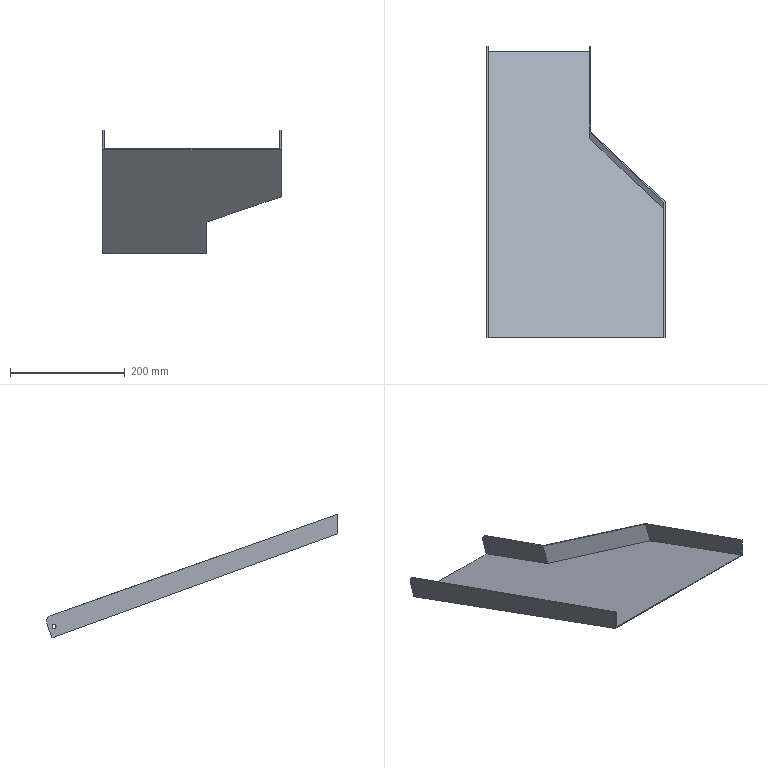Part | NX | features HB 2 | 1 solid | 18 faces | box 311 x 508.386 x 215.484 mm | volume 344938 mm3 | plane 14 | cylinder 4 | commonest cylinder face diameters 7 x2 20 x2
STEP:
#1=CARTESIAN_POINT('',(3094.,539.252,-364.707));
#2=VERTEX_POINT('',#1);
#3=CARTESIAN_POINT('',(3094.,691.161,-419.998));
#4=VERTEX_POINT('',#3);
#5=CARTESIAN_POINT('',(3094.,379.611,-306.603));
#6=DIRECTION('',(0.,0.9397,-0.342));
#7=VECTOR('',#6,1000.);
#8=LINE('',#5,#7);
#9=EDGE_CURVE('',#2,#4,#8,.T.);
#10=ORIENTED_EDGE('',*,*,#9,.T.);
#11=CARTESIAN_POINT('',(2917.,691.161,-419.998));
#12=VERTEX_POINT('',#11);
#13=CARTESIAN_POINT('',(2992.,691.161,-419.998));
#14=DIRECTION('',(1.,0.,0.));
#15=VECTOR('',#14,1000.);
#16=LINE('',#13,#15);
#17=EDGE_CURVE('',#12,#4,#16,.T.);
#18=ORIENTED_EDGE('',*,*,#17,.F.);
#19=CARTESIAN_POINT('',(2917.,192.,-238.318));
#20=VERTEX_POINT('',#19);
#21=CARTESIAN_POINT('',(2917.,379.611,-306.603));
#22=DIRECTION('',(0.,-0.9397,0.342));
#23=VECTOR('',#22,1000.);
#24=LINE('',#21,#23);
#25=EDGE_CURVE('',#12,#20,#24,.T.);
#26=ORIENTED_EDGE('',*,*,#25,.T.);
#27=CARTESIAN_POINT('',(3224.,192.,-238.318));
#28=VERTEX_POINT('',#27);
#29=CARTESIAN_POINT('',(2992.,192.,-238.318));
#30=DIRECTION('',(-1.,0.,0.));
#31=VECTOR('',#30,1000.);
#32=LINE('',#29,#31);
#33=EDGE_CURVE('',#28,#20,#32,.T.);
#34=ORIENTED_EDGE('',*,*,#33,.F.);
#35=CARTESIAN_POINT('',(3224.,417.092,-320.245));
#36=VERTEX_POINT('',#35);
#37=CARTESIAN_POINT('',(3224.,379.611,-306.603));
#38=DIRECTION('',(0.,0.9397,-0.342));
#39=VECTOR('',#38,1000.);
#40=LINE('',#37,#39);
#41=EDGE_CURVE('',#28,#36,#40,.T.);
#42=ORIENTED_EDGE('',*,*,#41,.T.);
#43=CARTESIAN_POINT('',(3127.943,507.356,-353.098));
#44=DIRECTION('',(-0.7071,0.6645,-0.2418));
#45=VECTOR('',#44,1000.);
#46=LINE('',#43,#45);
#47=EDGE_CURVE('',#36,#2,#46,.T.);
#48=ORIENTED_EDGE('',*,*,#47,.T.);
#49=EDGE_LOOP('',(#10,#18,#26,#34,#42,#48));
#50=FACE_BOUND('',#49,.T.);
#51=CARTESIAN_POINT('',(2992.,379.611,-306.603));
#52=DIRECTION('',(0.,0.342,0.9397));
#53=DIRECTION('',(1.,0.,0.));
#54=AXIS2_PLACEMENT_3D('',#51,#52,#53);
#55=PLANE('',#54);
#56=ADVANCED_FACE('',(#50),#55,.T.);
#57=ORIENTED_EDGE('',*,*,#33,.T.);
#58=CARTESIAN_POINT('',(2917.,192.,-206.393));
#59=VERTEX_POINT('',#58);
#60=CARTESIAN_POINT('',(2917.,192.,-306.603));
#61=DIRECTION('',(0.,0.,1.));
#62=VECTOR('',#61,1000.);
#63=LINE('',#60,#62);
#64=EDGE_CURVE('',#20,#59,#63,.T.);
#65=ORIENTED_EDGE('',*,*,#64,.T.);
#66=CARTESIAN_POINT('',(2915.,192.,-206.393));
#67=VERTEX_POINT('',#66);
#68=CARTESIAN_POINT('',(3433.,192.,-206.393));
#69=DIRECTION('',(1.,0.,0.));
#70=VECTOR('',#69,1000.);
#71=LINE('',#68,#70);
#72=EDGE_CURVE('',#67,#59,#71,.T.);
#73=ORIENTED_EDGE('',*,*,#72,.F.);
#74=CARTESIAN_POINT('',(2915.,192.,-240.446));
#75=VERTEX_POINT('',#74);
#76=CARTESIAN_POINT('',(2915.,192.,-306.603));
#77=DIRECTION('',(0.,0.,1.));
#78=VECTOR('',#77,1000.);
#79=LINE('',#76,#78);
#80=EDGE_CURVE('',#75,#67,#79,.T.);
#81=ORIENTED_EDGE('',*,*,#80,.F.);
#82=CARTESIAN_POINT('',(3226.,192.,-240.446));
#83=VERTEX_POINT('',#82);
#84=CARTESIAN_POINT('',(2992.,192.,-240.446));
#85=DIRECTION('',(-1.,0.,0.));
#86=VECTOR('',#85,1000.);
#87=LINE('',#84,#86);
#88=EDGE_CURVE('',#83,#75,#87,.T.);
#89=ORIENTED_EDGE('',*,*,#88,.F.);
#90=CARTESIAN_POINT('',(3226.,192.,-206.393));
#91=VERTEX_POINT('',#90);
#92=CARTESIAN_POINT('',(3226.,192.,-306.603));
#93=DIRECTION('',(0.,0.,-1.));
#94=VECTOR('',#93,1000.);
#95=LINE('',#92,#94);
#96=EDGE_CURVE('',#91,#83,#95,.T.);
#97=ORIENTED_EDGE('',*,*,#96,.F.);
#98=CARTESIAN_POINT('',(3224.,192.,-206.393));
#99=VERTEX_POINT('',#98);
#100=CARTESIAN_POINT('',(3433.,192.,-206.393));
#101=DIRECTION('',(1.,0.,0.));
#102=VECTOR('',#101,1000.);
#103=LINE('',#100,#102);
#104=EDGE_CURVE('',#99,#91,#103,.T.);
#105=ORIENTED_EDGE('',*,*,#104,.F.);
#106=CARTESIAN_POINT('',(3224.,192.,-306.603));
#107=DIRECTION('',(0.,0.,-1.));
#108=VECTOR('',#107,1000.);
#109=LINE('',#106,#108);
#110=EDGE_CURVE('',#99,#28,#109,.T.);
#111=ORIENTED_EDGE('',*,*,#110,.T.);
#112=EDGE_LOOP('',(#57,#65,#73,#81,#89,#97,#105,#111));
#113=FACE_BOUND('',#112,.T.);
#114=CARTESIAN_POINT('',(3433.,192.,70.));
#115=DIRECTION('',(0.,-1.,0.));
#116=DIRECTION('',(0.,0.,-1.));
#117=AXIS2_PLACEMENT_3D('',#114,#115,#116);
#118=PLANE('',#117);
#119=ADVANCED_FACE('',(#113),#118,.T.);
#120=CARTESIAN_POINT('',(3226.,417.186,-322.407));
#121=VERTEX_POINT('',#120);
#122=CARTESIAN_POINT('',(3096.,539.346,-366.87));
#123=VERTEX_POINT('',#122);
#124=CARTESIAN_POINT('',(3129.357,508.001,-355.461));
#125=DIRECTION('',(-0.7071,0.6645,-0.2418));
#126=VECTOR('',#125,1000.);
#127=LINE('',#124,#126);
#128=EDGE_CURVE('',#121,#123,#127,.T.);
#129=ORIENTED_EDGE('',*,*,#128,.F.);
#130=CARTESIAN_POINT('',(3226.,378.927,-308.482));
#131=DIRECTION('',(0.,-0.9397,0.342));
#132=VECTOR('',#131,1000.);
#133=LINE('',#130,#132);
#134=EDGE_CURVE('',#121,#83,#133,.T.);
#135=ORIENTED_EDGE('',*,*,#134,.T.);
#136=ORIENTED_EDGE('',*,*,#88,.T.);
#137=CARTESIAN_POINT('',(2915.,690.477,-421.877));
#138=VERTEX_POINT('',#137);
#139=CARTESIAN_POINT('',(2915.,378.927,-308.482));
#140=DIRECTION('',(0.,0.9397,-0.342));
#141=VECTOR('',#140,1000.);
#142=LINE('',#139,#141);
#143=EDGE_CURVE('',#75,#138,#142,.T.);
#144=ORIENTED_EDGE('',*,*,#143,.T.);
#145=CARTESIAN_POINT('',(3096.,690.477,-421.877));
#146=VERTEX_POINT('',#145);
#147=CARTESIAN_POINT('',(2992.,690.477,-421.877));
#148=DIRECTION('',(1.,0.,0.));
#149=VECTOR('',#148,1000.);
#150=LINE('',#147,#149);
#151=EDGE_CURVE('',#138,#146,#150,.T.);
#152=ORIENTED_EDGE('',*,*,#151,.T.);
#153=CARTESIAN_POINT('',(3096.,378.927,-308.482));
#154=DIRECTION('',(0.,-0.9397,0.342));
#155=VECTOR('',#154,1000.);
#156=LINE('',#153,#155);
#157=EDGE_CURVE('',#146,#123,#156,.T.);
#158=ORIENTED_EDGE('',*,*,#157,.T.);
#159=EDGE_LOOP('',(#129,#135,#136,#144,#152,#158));
#160=FACE_BOUND('',#159,.T.);
#161=CARTESIAN_POINT('',(2992.,378.927,-308.482));
#162=DIRECTION('',(0.,0.342,0.9397));
#163=DIRECTION('',(1.,0.,0.));
#164=AXIS2_PLACEMENT_3D('',#161,#162,#163);
#165=PLANE('',#164);
#166=ADVANCED_FACE('',(#160),#165,.F.);
#167=CARTESIAN_POINT('',(2915.,693.714,-383.458));
#168=VERTEX_POINT('',#167);
#169=CARTESIAN_POINT('',(2915.,390.558,-276.468));
#170=DIRECTION('',(0.,-0.943,0.3328));
#171=VECTOR('',#170,1000.);
#172=LINE('',#169,#171);
#173=EDGE_CURVE('',#168,#67,#172,.T.);
#174=ORIENTED_EDGE('',*,*,#173,.T.);
#175=ORIENTED_EDGE('',*,*,#72,.T.);
#176=CARTESIAN_POINT('',(2917.,693.714,-383.458));
#177=VERTEX_POINT('',#176);
#178=CARTESIAN_POINT('',(2917.,390.558,-276.468));
#179=DIRECTION('',(0.,-0.943,0.3328));
#180=VECTOR('',#179,1000.);
#181=LINE('',#178,#180);
#182=EDGE_CURVE('',#177,#59,#181,.T.);
#183=ORIENTED_EDGE('',*,*,#182,.F.);
#184=CARTESIAN_POINT('',(2992.,693.714,-383.458));
#185=DIRECTION('',(1.,0.,0.));
#186=VECTOR('',#185,1000.);
#187=LINE('',#184,#186);
#188=EDGE_CURVE('',#168,#177,#187,.T.);
#189=ORIENTED_EDGE('',*,*,#188,.F.);
#190=EDGE_LOOP('',(#174,#175,#183,#189));
#191=FACE_BOUND('',#190,.T.);
#192=CARTESIAN_POINT('',(2927.,390.558,-276.468));
#193=DIRECTION('',(0.,-0.3328,-0.943));
#194=DIRECTION('',(0.,0.943,-0.3328));
#195=AXIS2_PLACEMENT_3D('',#192,#193,#194);
#196=PLANE('',#195);
#197=ADVANCED_FACE('',(#191),#196,.F.);
#198=ORIENTED_EDGE('',*,*,#182,.T.);
#199=ORIENTED_EDGE('',*,*,#64,.F.);
#200=ORIENTED_EDGE('',*,*,#25,.F.);
#201=CARTESIAN_POINT('',(2917.,699.783,-396.309));
#202=VERTEX_POINT('',#201);
#203=CARTESIAN_POINT('',(2917.,692.943,-415.102));
#204=DIRECTION('',(0.,0.342,0.9397));
#205=VECTOR('',#204,1000.);
#206=LINE('',#203,#205);
#207=EDGE_CURVE('',#12,#202,#206,.T.);
#208=ORIENTED_EDGE('',*,*,#207,.T.);
#209=CARTESIAN_POINT('',(2917.,690.386,-392.888));
#210=DIRECTION('',(-1.,0.,0.));
#211=DIRECTION('',(0.,0.,-1.));
#212=AXIS2_PLACEMENT_3D('',#209,#210,#211);
#213=CIRCLE('',#212,10.);
#214=EDGE_CURVE('',#177,#202,#213,.T.);
#215=ORIENTED_EDGE('',*,*,#214,.F.);
#216=EDGE_LOOP('',(#198,#199,#200,#208,#215));
#217=FACE_BOUND('',#216,.T.);
#218=CARTESIAN_POINT('',(2917.,686.661,-398.799));
#219=VERTEX_POINT('',#218);
#220=CARTESIAN_POINT('',(2917.,686.966,-402.285));
#221=DIRECTION('',(1.,0.,0.));
#222=DIRECTION('',(0.,-0.08716,0.9962));
#223=AXIS2_PLACEMENT_3D('',#220,#221,#222);
#224=CIRCLE('',#223,3.5);
#225=EDGE_CURVE('',#219,#219,#224,.T.);
#226=ORIENTED_EDGE('',*,*,#225,.F.);
#227=EDGE_LOOP('',(#226));
#228=FACE_BOUND('',#227,.T.);
#229=CARTESIAN_POINT('',(2917.,379.611,-306.603));
#230=DIRECTION('',(1.,0.,0.));
#231=DIRECTION('',(0.,-0.08716,0.9962));
#232=AXIS2_PLACEMENT_3D('',#229,#230,#231);
#233=PLANE('',#232);
#234=ADVANCED_FACE('',(#217,#228),#233,.T.);
#235=CARTESIAN_POINT('',(3096.,551.568,-333.292));
#236=VERTEX_POINT('',#235);
#237=CARTESIAN_POINT('',(3226.,428.973,-290.025));
#238=VERTEX_POINT('',#237);
#239=CARTESIAN_POINT('',(3226.012,428.961,-290.021));
#240=DIRECTION('',(0.7071,-0.6668,0.2353));
#241=VECTOR('',#240,1000.);
#242=LINE('',#239,#241);
#243=EDGE_CURVE('',#236,#238,#242,.T.);
#244=ORIENTED_EDGE('',*,*,#243,.F.);
#245=CARTESIAN_POINT('',(3096.,693.714,-383.458));
#246=VERTEX_POINT('',#245);
#247=CARTESIAN_POINT('',(3096.,390.558,-276.468));
#248=DIRECTION('',(0.,-0.943,0.3328));
#249=VECTOR('',#248,1000.);
#250=LINE('',#247,#249);
#251=EDGE_CURVE('',#246,#236,#250,.T.);
#252=ORIENTED_EDGE('',*,*,#251,.F.);
#253=CARTESIAN_POINT('',(3094.,693.714,-383.458));
#254=VERTEX_POINT('',#253);
#255=CARTESIAN_POINT('',(3224.,693.714,-383.458));
#256=DIRECTION('',(1.,0.,0.));
#257=VECTOR('',#256,1000.);
#258=LINE('',#255,#257);
#259=EDGE_CURVE('',#254,#246,#258,.T.);
#260=ORIENTED_EDGE('',*,*,#259,.F.);
#261=CARTESIAN_POINT('',(3094.,550.787,-333.016));
#262=VERTEX_POINT('',#261);
#263=CARTESIAN_POINT('',(3094.,390.558,-276.468));
#264=DIRECTION('',(0.,-0.943,0.3328));
#265=VECTOR('',#264,1000.);
#266=LINE('',#263,#265);
#267=EDGE_CURVE('',#254,#262,#266,.T.);
#268=ORIENTED_EDGE('',*,*,#267,.T.);
#269=CARTESIAN_POINT('',(3224.,428.191,-289.75));
#270=VERTEX_POINT('',#269);
#271=CARTESIAN_POINT('',(3224.598,427.628,-289.551));
#272=DIRECTION('',(0.7071,-0.6668,0.2353));
#273=VECTOR('',#272,1000.);
#274=LINE('',#271,#273);
#275=EDGE_CURVE('',#262,#270,#274,.T.);
#276=ORIENTED_EDGE('',*,*,#275,.T.);
#277=CARTESIAN_POINT('',(3224.,390.558,-276.468));
#278=DIRECTION('',(0.,-0.943,0.3328));
#279=VECTOR('',#278,1000.);
#280=LINE('',#277,#279);
#281=EDGE_CURVE('',#270,#99,#280,.T.);
#282=ORIENTED_EDGE('',*,*,#281,.T.);
#283=ORIENTED_EDGE('',*,*,#104,.T.);
#284=CARTESIAN_POINT('',(3226.,390.558,-276.468));
#285=DIRECTION('',(0.,-0.943,0.3328));
#286=VECTOR('',#285,1000.);
#287=LINE('',#284,#286);
#288=EDGE_CURVE('',#238,#91,#287,.T.);
#289=ORIENTED_EDGE('',*,*,#288,.F.);
#290=EDGE_LOOP('',(#244,#252,#260,#268,#276,#282,#283,#289));
#291=FACE_BOUND('',#290,.T.);
#292=CARTESIAN_POINT('',(3224.,390.558,-276.468));
#293=DIRECTION('',(0.,-0.3328,-0.943));
#294=DIRECTION('',(0.,0.943,-0.3328));
#295=AXIS2_PLACEMENT_3D('',#292,#293,#294);
#296=PLANE('',#295);
#297=ADVANCED_FACE('',(#291),#296,.F.);
#298=CARTESIAN_POINT('',(3224.,417.092,-320.245));
#299=DIRECTION('',(0.,-0.342,-0.9397));
#300=VECTOR('',#299,1000.);
#301=LINE('',#298,#300);
#302=EDGE_CURVE('',#270,#36,#301,.T.);
#303=ORIENTED_EDGE('',*,*,#302,.T.);
#304=ORIENTED_EDGE('',*,*,#41,.F.);
#305=ORIENTED_EDGE('',*,*,#110,.F.);
#306=ORIENTED_EDGE('',*,*,#281,.F.);
#307=EDGE_LOOP('',(#303,#304,#305,#306));
#308=FACE_BOUND('',#307,.T.);
#309=CARTESIAN_POINT('',(3224.,379.611,-306.603));
#310=DIRECTION('',(-1.,0.,0.));
#311=DIRECTION('',(0.,-0.08716,0.9962));
#312=AXIS2_PLACEMENT_3D('',#309,#310,#311);
#313=PLANE('',#312);
#314=ADVANCED_FACE('',(#308),#313,.T.);
#315=ORIENTED_EDGE('',*,*,#288,.T.);
#316=ORIENTED_EDGE('',*,*,#96,.T.);
#317=ORIENTED_EDGE('',*,*,#134,.F.);
#318=CARTESIAN_POINT('',(3226.,417.87,-320.528));
#319=DIRECTION('',(0.,0.342,0.9397));
#320=VECTOR('',#319,1000.);
#321=LINE('',#318,#320);
#322=EDGE_CURVE('',#121,#238,#321,.T.);
#323=ORIENTED_EDGE('',*,*,#322,.T.);
#324=EDGE_LOOP('',(#315,#316,#317,#323));
#325=FACE_BOUND('',#324,.T.);
#326=CARTESIAN_POINT('',(3226.,379.611,-306.603));
#327=DIRECTION('',(-1.,0.,0.));
#328=DIRECTION('',(0.,-0.08716,0.9962));
#329=AXIS2_PLACEMENT_3D('',#326,#327,#328);
#330=PLANE('',#329);
#331=ADVANCED_FACE('',(#325),#330,.F.);
#332=ORIENTED_EDGE('',*,*,#143,.F.);
#333=ORIENTED_EDGE('',*,*,#80,.T.);
#334=ORIENTED_EDGE('',*,*,#173,.F.);
#335=CARTESIAN_POINT('',(2915.,699.783,-396.309));
#336=VERTEX_POINT('',#335);
#337=CARTESIAN_POINT('',(2915.,690.386,-392.888));
#338=DIRECTION('',(1.,0.,0.));
#339=DIRECTION('',(0.,0.,-1.));
#340=AXIS2_PLACEMENT_3D('',#337,#338,#339);
#341=CIRCLE('',#340,10.);
#342=EDGE_CURVE('',#336,#168,#341,.T.);
#343=ORIENTED_EDGE('',*,*,#342,.F.);
#344=CARTESIAN_POINT('',(2915.,692.943,-415.102));
#345=DIRECTION('',(0.,0.342,0.9397));
#346=VECTOR('',#345,1000.);
#347=LINE('',#344,#346);
#348=EDGE_CURVE('',#138,#336,#347,.T.);
#349=ORIENTED_EDGE('',*,*,#348,.F.);
#350=EDGE_LOOP('',(#332,#333,#334,#343,#349));
#351=FACE_BOUND('',#350,.T.);
#352=CARTESIAN_POINT('',(2915.,686.661,-398.799));
#353=VERTEX_POINT('',#352);
#354=CARTESIAN_POINT('',(2915.,686.966,-402.285));
#355=DIRECTION('',(1.,0.,0.));
#356=DIRECTION('',(0.,-0.08716,0.9962));
#357=AXIS2_PLACEMENT_3D('',#354,#355,#356);
#358=CIRCLE('',#357,3.5);
#359=EDGE_CURVE('',#353,#353,#358,.T.);
#360=ORIENTED_EDGE('',*,*,#359,.T.);
#361=EDGE_LOOP('',(#360));
#362=FACE_BOUND('',#361,.T.);
#363=CARTESIAN_POINT('',(2915.,379.611,-306.603));
#364=DIRECTION('',(1.,0.,0.));
#365=DIRECTION('',(0.,0.08716,-0.9962));
#366=AXIS2_PLACEMENT_3D('',#363,#364,#365);
#367=PLANE('',#366);
#368=ADVANCED_FACE('',(#351,#362),#367,.F.);
#369=CARTESIAN_POINT('',(3096.,687.271,-405.772));
#370=VERTEX_POINT('',#369);
#371=CARTESIAN_POINT('',(3096.,686.966,-402.285));
#372=DIRECTION('',(1.,0.,0.));
#373=DIRECTION('',(0.,0.08716,-0.9962));
#374=AXIS2_PLACEMENT_3D('',#371,#372,#373);
#375=CIRCLE('',#374,3.5);
#376=EDGE_CURVE('',#370,#370,#375,.T.);
#377=ORIENTED_EDGE('',*,*,#376,.F.);
#378=EDGE_LOOP('',(#377));
#379=FACE_BOUND('',#378,.T.);
#380=ORIENTED_EDGE('',*,*,#157,.F.);
#381=CARTESIAN_POINT('',(3096.,699.783,-396.309));
#382=VERTEX_POINT('',#381);
#383=CARTESIAN_POINT('',(3096.,692.943,-415.102));
#384=DIRECTION('',(0.,0.342,0.9397));
#385=VECTOR('',#384,1000.);
#386=LINE('',#383,#385);
#387=EDGE_CURVE('',#146,#382,#386,.T.);
#388=ORIENTED_EDGE('',*,*,#387,.T.);
#389=CARTESIAN_POINT('',(3096.,690.386,-392.888));
#390=DIRECTION('',(-1.,0.,0.));
#391=DIRECTION('',(0.,0.,1.));
#392=AXIS2_PLACEMENT_3D('',#389,#390,#391);
#393=CIRCLE('',#392,10.);
#394=EDGE_CURVE('',#246,#382,#393,.T.);
#395=ORIENTED_EDGE('',*,*,#394,.F.);
#396=ORIENTED_EDGE('',*,*,#251,.T.);
#397=CARTESIAN_POINT('',(3096.,540.03,-364.991));
#398=DIRECTION('',(0.,0.342,0.9397));
#399=VECTOR('',#398,1000.);
#400=LINE('',#397,#399);
#401=EDGE_CURVE('',#123,#236,#400,.T.);
#402=ORIENTED_EDGE('',*,*,#401,.F.);
#403=EDGE_LOOP('',(#380,#388,#395,#396,#402));
#404=FACE_BOUND('',#403,.T.);
#405=CARTESIAN_POINT('',(3096.,379.611,-306.603));
#406=DIRECTION('',(-1.,0.,0.));
#407=DIRECTION('',(0.,-0.08716,0.9962));
#408=AXIS2_PLACEMENT_3D('',#405,#406,#407);
#409=PLANE('',#408);
#410=ADVANCED_FACE('',(#379,#404),#409,.F.);
#411=CARTESIAN_POINT('',(3094.,687.271,-405.772));
#412=VERTEX_POINT('',#411);
#413=CARTESIAN_POINT('',(3094.,686.966,-402.285));
#414=DIRECTION('',(-1.,0.,0.));
#415=DIRECTION('',(0.,0.08716,-0.9962));
#416=AXIS2_PLACEMENT_3D('',#413,#414,#415);
#417=CIRCLE('',#416,3.5);
#418=EDGE_CURVE('',#412,#412,#417,.T.);
#419=ORIENTED_EDGE('',*,*,#418,.F.);
#420=EDGE_LOOP('',(#419));
#421=FACE_BOUND('',#420,.T.);
#422=ORIENTED_EDGE('',*,*,#267,.F.);
#423=CARTESIAN_POINT('',(3094.,699.783,-396.309));
#424=VERTEX_POINT('',#423);
#425=CARTESIAN_POINT('',(3094.,690.386,-392.888));
#426=DIRECTION('',(1.,0.,0.));
#427=DIRECTION('',(0.,0.,1.));
#428=AXIS2_PLACEMENT_3D('',#425,#426,#427);
#429=CIRCLE('',#428,10.);
#430=EDGE_CURVE('',#424,#254,#429,.T.);
#431=ORIENTED_EDGE('',*,*,#430,.F.);
#432=CARTESIAN_POINT('',(3094.,692.943,-415.102));
#433=DIRECTION('',(0.,0.342,0.9397));
#434=VECTOR('',#433,1000.);
#435=LINE('',#432,#434);
#436=EDGE_CURVE('',#4,#424,#435,.T.);
#437=ORIENTED_EDGE('',*,*,#436,.F.);
#438=ORIENTED_EDGE('',*,*,#9,.F.);
#439=CARTESIAN_POINT('',(3094.,539.252,-364.707));
#440=DIRECTION('',(0.,0.342,0.9397));
#441=VECTOR('',#440,1000.);
#442=LINE('',#439,#441);
#443=EDGE_CURVE('',#2,#262,#442,.T.);
#444=ORIENTED_EDGE('',*,*,#443,.T.);
#445=EDGE_LOOP('',(#422,#431,#437,#438,#444));
#446=FACE_BOUND('',#445,.T.);
#447=CARTESIAN_POINT('',(3094.,379.611,-306.603));
#448=DIRECTION('',(-1.,0.,0.));
#449=DIRECTION('',(0.,-0.08716,0.9962));
#450=AXIS2_PLACEMENT_3D('',#447,#448,#449);
#451=PLANE('',#450);
#452=ADVANCED_FACE('',(#421,#446),#451,.T.);
#453=ORIENTED_EDGE('',*,*,#348,.T.);
#454=CARTESIAN_POINT('',(2992.,699.783,-396.309));
#455=DIRECTION('',(-1.,0.,0.));
#456=VECTOR('',#455,1000.);
#457=LINE('',#454,#456);
#458=EDGE_CURVE('',#202,#336,#457,.T.);
#459=ORIENTED_EDGE('',*,*,#458,.F.);
#460=ORIENTED_EDGE('',*,*,#207,.F.);
#461=ORIENTED_EDGE('',*,*,#17,.T.);
#462=ORIENTED_EDGE('',*,*,#436,.T.);
#463=CARTESIAN_POINT('',(3224.,699.783,-396.309));
#464=DIRECTION('',(-1.,0.,0.));
#465=VECTOR('',#464,1000.);
#466=LINE('',#463,#465);
#467=EDGE_CURVE('',#382,#424,#466,.T.);
#468=ORIENTED_EDGE('',*,*,#467,.F.);
#469=ORIENTED_EDGE('',*,*,#387,.F.);
#470=ORIENTED_EDGE('',*,*,#151,.F.);
#471=EDGE_LOOP('',(#453,#459,#460,#461,#462,#468,#469,#470));
#472=FACE_BOUND('',#471,.T.);
#473=CARTESIAN_POINT('',(2992.,692.943,-415.102));
#474=DIRECTION('',(0.,-0.9397,0.342));
#475=DIRECTION('',(0.,-0.342,-0.9397));
#476=AXIS2_PLACEMENT_3D('',#473,#474,#475);
#477=PLANE('',#476);
#478=ADVANCED_FACE('',(#472),#477,.F.);
#479=ORIENTED_EDGE('',*,*,#214,.T.);
#480=ORIENTED_EDGE('',*,*,#458,.T.);
#481=ORIENTED_EDGE('',*,*,#342,.T.);
#482=ORIENTED_EDGE('',*,*,#188,.T.);
#483=EDGE_LOOP('',(#479,#480,#481,#482));
#484=FACE_BOUND('',#483,.T.);
#485=CARTESIAN_POINT('',(2992.,690.386,-392.888));
#486=DIRECTION('',(1.,0.,0.));
#487=DIRECTION('',(0.,0.,1.));
#488=AXIS2_PLACEMENT_3D('',#485,#486,#487);
#489=CYLINDRICAL_SURFACE('',#488,10.);
#490=ADVANCED_FACE('',(#484),#489,.T.);
#491=ORIENTED_EDGE('',*,*,#430,.T.);
#492=ORIENTED_EDGE('',*,*,#259,.T.);
#493=ORIENTED_EDGE('',*,*,#394,.T.);
#494=ORIENTED_EDGE('',*,*,#467,.T.);
#495=EDGE_LOOP('',(#491,#492,#493,#494));
#496=FACE_BOUND('',#495,.T.);
#497=CARTESIAN_POINT('',(3224.,690.386,-392.888));
#498=DIRECTION('',(-1.,0.,0.));
#499=DIRECTION('',(0.,0.,-1.));
#500=AXIS2_PLACEMENT_3D('',#497,#498,#499);
#501=CYLINDRICAL_SURFACE('',#500,10.);
#502=ADVANCED_FACE('',(#496),#501,.T.);
#503=ORIENTED_EDGE('',*,*,#225,.T.);
#504=EDGE_LOOP('',(#503));
#505=FACE_BOUND('',#504,.T.);
#506=ORIENTED_EDGE('',*,*,#359,.F.);
#507=EDGE_LOOP('',(#506));
#508=FACE_BOUND('',#507,.T.);
#509=CARTESIAN_POINT('',(2323.,686.966,-402.285));
#510=DIRECTION('',(1.,0.,0.));
#511=DIRECTION('',(0.,0.08716,-0.9962));
#512=AXIS2_PLACEMENT_3D('',#509,#510,#511);
#513=CYLINDRICAL_SURFACE('',#512,3.5);
#514=ADVANCED_FACE('',(#505,#508),#513,.F.);
#515=ORIENTED_EDGE('',*,*,#418,.T.);
#516=EDGE_LOOP('',(#515));
#517=FACE_BOUND('',#516,.T.);
#518=ORIENTED_EDGE('',*,*,#376,.T.);
#519=EDGE_LOOP('',(#518));
#520=FACE_BOUND('',#519,.T.);
#521=CARTESIAN_POINT('',(2374.,686.966,-402.285));
#522=DIRECTION('',(1.,0.,0.));
#523=DIRECTION('',(0.,0.08716,-0.9962));
#524=AXIS2_PLACEMENT_3D('',#521,#522,#523);
#525=CYLINDRICAL_SURFACE('',#524,3.5);
#526=ADVANCED_FACE('',(#517,#520),#525,.F.);
#527=ORIENTED_EDGE('',*,*,#401,.T.);
#528=ORIENTED_EDGE('',*,*,#243,.T.);
#529=ORIENTED_EDGE('',*,*,#322,.F.);
#530=ORIENTED_EDGE('',*,*,#128,.T.);
#531=EDGE_LOOP('',(#527,#528,#529,#530));
#532=FACE_BOUND('',#531,.T.);
#533=CARTESIAN_POINT('',(3226.,428.131,-292.337));
#534=DIRECTION('',(0.7071,0.6645,-0.2418));
#535=DIRECTION('',(0.,-0.342,-0.9397));
#536=AXIS2_PLACEMENT_3D('',#533,#534,#535);
#537=PLANE('',#536);
#538=ADVANCED_FACE('',(#532),#537,.T.);
#539=ORIENTED_EDGE('',*,*,#302,.F.);
#540=ORIENTED_EDGE('',*,*,#275,.F.);
#541=ORIENTED_EDGE('',*,*,#443,.F.);
#542=ORIENTED_EDGE('',*,*,#47,.F.);
#543=EDGE_LOOP('',(#539,#540,#541,#542));
#544=FACE_BOUND('',#543,.T.);
#545=CARTESIAN_POINT('',(3224.586,426.802,-291.854));
#546=DIRECTION('',(0.7071,0.6645,-0.2418));
#547=DIRECTION('',(0.,-0.342,-0.9397));
#548=AXIS2_PLACEMENT_3D('',#545,#546,#547);
#549=PLANE('',#548);
#550=ADVANCED_FACE('',(#544),#549,.F.);
#551=CLOSED_SHELL('',(#56,#119,#166,#197,#234,#297,#314,#331,#368,#410,#452,#478,#490,#502,#514,#526,#538,#550));
#552=MANIFOLD_SOLID_BREP('',#551);
#553=(LENGTH_UNIT()NAMED_UNIT(*)SI_UNIT(.MILLI.,.METRE.));
#554=UNCERTAINTY_MEASURE_WITH_UNIT(LENGTH_MEASURE(0.00001),#553,'','');
#555=(NAMED_UNIT(*)PLANE_ANGLE_UNIT()SI_UNIT($,.RADIAN.));
#556=(NAMED_UNIT(*)SI_UNIT($,.STERADIAN.)SOLID_ANGLE_UNIT());
#557=(GEOMETRIC_REPRESENTATION_CONTEXT(3)GLOBAL_UNCERTAINTY_ASSIGNED_CONTEXT((#554))GLOBAL_UNIT_ASSIGNED_CONTEXT((#553,#555,#556))REPRESENTATION_CONTEXT('',''));
#558=ADVANCED_BREP_SHAPE_REPRESENTATION('',(#552),#557);